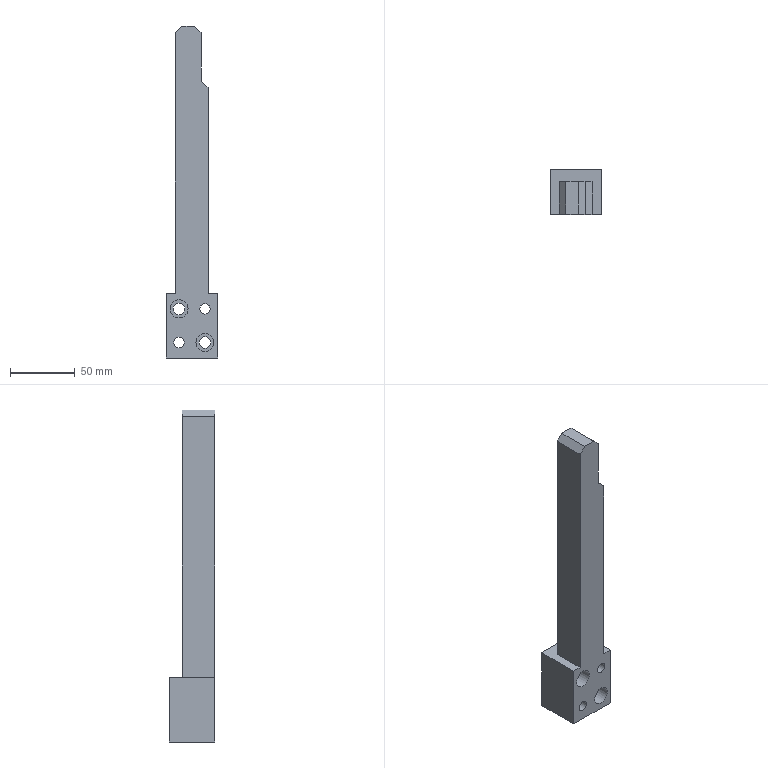Part | STEP file | 车灯-后视镜_id162_x_t | 1 solid | 24 faces | box 40 x 35 x 257 mm | volume 187577 mm3 | plane 16 | cylinder 8 | commonest cylinder face diameters 4 x2 8 x2 9 x2 14 x2
STEP:
#1=CARTESIAN_POINT('',(64.914,-310.,-210.914));
#2=VERTEX_POINT('',#1);
#3=CARTESIAN_POINT('',(60.086,-310.,-206.086));
#4=VERTEX_POINT('',#3);
#5=CARTESIAN_POINT('',(65.5,-310.,-211.5));
#6=DIRECTION('',(-0.7071,0.,0.7071));
#7=VECTOR('',#6,1.);
#8=LINE('',#5,#7);
#9=EDGE_CURVE('',#2,#4,#8,.T.);
#10=ORIENTED_EDGE('',*,*,#9,.F.);
#11=CARTESIAN_POINT('',(64.914,-285.,-210.914));
#12=VERTEX_POINT('',#11);
#13=CARTESIAN_POINT('',(64.914,-285.,-210.914));
#14=DIRECTION('',(0.,1.,0.));
#15=VECTOR('',#14,1.);
#16=LINE('',#13,#15);
#17=EDGE_CURVE('',#2,#12,#16,.T.);
#18=ORIENTED_EDGE('',*,*,#17,.T.);
#19=CARTESIAN_POINT('',(60.086,-285.,-206.086));
#20=VERTEX_POINT('',#19);
#21=CARTESIAN_POINT('',(65.5,-285.,-211.5));
#22=DIRECTION('',(0.7071,0.,-0.7071));
#23=VECTOR('',#22,1.);
#24=LINE('',#21,#23);
#25=EDGE_CURVE('',#20,#12,#24,.T.);
#26=ORIENTED_EDGE('',*,*,#25,.F.);
#27=CARTESIAN_POINT('',(60.086,-310.,-206.086));
#28=DIRECTION('',(0.,-1.,0.));
#29=VECTOR('',#28,1.);
#30=LINE('',#27,#29);
#31=EDGE_CURVE('',#20,#4,#30,.T.);
#32=ORIENTED_EDGE('',*,*,#31,.T.);
#33=EDGE_LOOP('',(#10,#18,#26,#32));
#34=FACE_OUTER_BOUND('',#33,.T.);
#35=CARTESIAN_POINT('',(65.5,-285.,-211.5));
#36=DIRECTION('',(0.7071,0.,0.7071));
#37=DIRECTION('',(0.7071,0.,-0.7071));
#38=AXIS2_PLACEMENT_3D('',#35,#36,#37);
#39=PLANE('',#38);
#40=ADVANCED_FACE('',(#34),#39,.T.);
#41=CARTESIAN_POINT('',(65.5,-285.,-370.5));
#42=VERTEX_POINT('',#41);
#43=CARTESIAN_POINT('',(65.5,-285.,-212.328));
#44=VERTEX_POINT('',#43);
#45=CARTESIAN_POINT('',(65.5,-285.,-420.5));
#46=DIRECTION('',(0.,0.,1.));
#47=VECTOR('',#46,1.);
#48=LINE('',#45,#47);
#49=EDGE_CURVE('',#42,#44,#48,.T.);
#50=ORIENTED_EDGE('',*,*,#49,.T.);
#51=CARTESIAN_POINT('',(65.5,-310.,-212.328));
#52=VERTEX_POINT('',#51);
#53=CARTESIAN_POINT('',(65.5,-292.5,-212.328));
#54=DIRECTION('',(0.,-1.,0.));
#55=VECTOR('',#54,1.);
#56=LINE('',#53,#55);
#57=EDGE_CURVE('',#44,#52,#56,.T.);
#58=ORIENTED_EDGE('',*,*,#57,.T.);
#59=CARTESIAN_POINT('',(65.5,-310.,-370.5));
#60=VERTEX_POINT('',#59);
#61=CARTESIAN_POINT('',(65.5,-310.,-420.5));
#62=DIRECTION('',(0.,0.,1.));
#63=VECTOR('',#62,1.);
#64=LINE('',#61,#63);
#65=EDGE_CURVE('',#60,#52,#64,.T.);
#66=ORIENTED_EDGE('',*,*,#65,.F.);
#67=CARTESIAN_POINT('',(65.5,-292.5,-370.5));
#68=DIRECTION('',(0.,1.,0.));
#69=VECTOR('',#68,1.);
#70=LINE('',#67,#69);
#71=EDGE_CURVE('',#60,#42,#70,.T.);
#72=ORIENTED_EDGE('',*,*,#71,.T.);
#73=EDGE_LOOP('',(#50,#58,#66,#72));
#74=FACE_OUTER_BOUND('',#73,.T.);
#75=CARTESIAN_POINT('',(65.5,-292.5,-420.5));
#76=DIRECTION('',(1.,0.,0.));
#77=DIRECTION('',(0.,0.,-1.));
#78=AXIS2_PLACEMENT_3D('',#75,#76,#77);
#79=PLANE('',#78);
#80=ADVANCED_FACE('',(#74),#79,.T.);
#81=ORIENTED_EDGE('',*,*,#25,.T.);
#82=CARTESIAN_POINT('',(63.5,-285.,-212.328));
#83=DIRECTION('',(0.,1.,0.));
#84=DIRECTION('',(0.,0.,1.));
#85=AXIS2_PLACEMENT_3D('',#82,#83,#84);
#86=CIRCLE('',#85,2.);
#87=EDGE_CURVE('',#12,#44,#86,.T.);
#88=ORIENTED_EDGE('',*,*,#87,.T.);
#89=ORIENTED_EDGE('',*,*,#49,.F.);
#90=CARTESIAN_POINT('',(39.5,-285.,-370.5));
#91=VERTEX_POINT('',#90);
#92=CARTESIAN_POINT('',(52.5,-285.,-370.5));
#93=DIRECTION('',(-1.,0.,0.));
#94=VECTOR('',#93,1.);
#95=LINE('',#92,#94);
#96=EDGE_CURVE('',#42,#91,#95,.T.);
#97=ORIENTED_EDGE('',*,*,#96,.T.);
#98=CARTESIAN_POINT('',(39.5,-285.,-168.5));
#99=VERTEX_POINT('',#98);
#100=CARTESIAN_POINT('',(39.5,-285.,-420.5));
#101=DIRECTION('',(0.,0.,1.));
#102=VECTOR('',#101,1.);
#103=LINE('',#100,#102);
#104=EDGE_CURVE('',#91,#99,#103,.T.);
#105=ORIENTED_EDGE('',*,*,#104,.T.);
#106=CARTESIAN_POINT('',(44.5,-285.,-163.5));
#107=VERTEX_POINT('',#106);
#108=CARTESIAN_POINT('',(39.5,-285.,-168.5));
#109=DIRECTION('',(0.7071,0.,0.7071));
#110=VECTOR('',#109,1.);
#111=LINE('',#108,#110);
#112=EDGE_CURVE('',#99,#107,#111,.T.);
#113=ORIENTED_EDGE('',*,*,#112,.T.);
#114=CARTESIAN_POINT('',(54.5,-285.,-163.5));
#115=VERTEX_POINT('',#114);
#116=CARTESIAN_POINT('',(52.5,-285.,-163.5));
#117=DIRECTION('',(1.,0.,0.));
#118=VECTOR('',#117,1.);
#119=LINE('',#116,#118);
#120=EDGE_CURVE('',#107,#115,#119,.T.);
#121=ORIENTED_EDGE('',*,*,#120,.T.);
#122=CARTESIAN_POINT('',(59.5,-285.,-168.5));
#123=VERTEX_POINT('',#122);
#124=CARTESIAN_POINT('',(59.5,-285.,-168.5));
#125=DIRECTION('',(0.7071,0.,-0.7071));
#126=VECTOR('',#125,1.);
#127=LINE('',#124,#126);
#128=EDGE_CURVE('',#115,#123,#127,.T.);
#129=ORIENTED_EDGE('',*,*,#128,.T.);
#130=CARTESIAN_POINT('',(59.5,-285.,-204.672));
#131=VERTEX_POINT('',#130);
#132=CARTESIAN_POINT('',(59.5,-285.,-420.5));
#133=DIRECTION('',(0.,0.,1.));
#134=VECTOR('',#133,1.);
#135=LINE('',#132,#134);
#136=EDGE_CURVE('',#131,#123,#135,.T.);
#137=ORIENTED_EDGE('',*,*,#136,.F.);
#138=CARTESIAN_POINT('',(61.5,-285.,-204.672));
#139=DIRECTION('',(0.,-1.,0.));
#140=DIRECTION('',(0.,0.,1.));
#141=AXIS2_PLACEMENT_3D('',#138,#139,#140);
#142=CIRCLE('',#141,2.);
#143=EDGE_CURVE('',#131,#20,#142,.T.);
#144=ORIENTED_EDGE('',*,*,#143,.T.);
#145=EDGE_LOOP('',(#81,#88,#89,#97,#105,#113,#121,#129,#137,#144));
#146=FACE_OUTER_BOUND('',#145,.T.);
#147=CARTESIAN_POINT('',(52.5,-285.,-420.5));
#148=DIRECTION('',(0.,1.,0.));
#149=DIRECTION('',(0.,0.,1.));
#150=AXIS2_PLACEMENT_3D('',#147,#148,#149);
#151=PLANE('',#150);
#152=ADVANCED_FACE('',(#146),#151,.T.);
#153=CARTESIAN_POINT('',(39.5,-310.,-370.5));
#154=VERTEX_POINT('',#153);
#155=CARTESIAN_POINT('',(39.5,-310.,-168.5));
#156=VERTEX_POINT('',#155);
#157=CARTESIAN_POINT('',(39.5,-310.,-420.5));
#158=DIRECTION('',(0.,0.,1.));
#159=VECTOR('',#158,1.);
#160=LINE('',#157,#159);
#161=EDGE_CURVE('',#154,#156,#160,.T.);
#162=ORIENTED_EDGE('',*,*,#161,.T.);
#163=CARTESIAN_POINT('',(39.5,-292.5,-168.5));
#164=DIRECTION('',(0.,1.,0.));
#165=VECTOR('',#164,1.);
#166=LINE('',#163,#165);
#167=EDGE_CURVE('',#156,#99,#166,.T.);
#168=ORIENTED_EDGE('',*,*,#167,.T.);
#169=ORIENTED_EDGE('',*,*,#104,.F.);
#170=CARTESIAN_POINT('',(39.5,-292.5,-370.5));
#171=DIRECTION('',(0.,-1.,0.));
#172=VECTOR('',#171,1.);
#173=LINE('',#170,#172);
#174=EDGE_CURVE('',#91,#154,#173,.T.);
#175=ORIENTED_EDGE('',*,*,#174,.T.);
#176=EDGE_LOOP('',(#162,#168,#169,#175));
#177=FACE_OUTER_BOUND('',#176,.T.);
#178=CARTESIAN_POINT('',(39.5,-292.5,-420.5));
#179=DIRECTION('',(-1.,0.,0.));
#180=DIRECTION('',(0.,0.,1.));
#181=AXIS2_PLACEMENT_3D('',#178,#179,#180);
#182=PLANE('',#181);
#183=ADVANCED_FACE('',(#177),#182,.T.);
#184=CARTESIAN_POINT('',(55.5,-310.,-408.5));
#185=VERTEX_POINT('',#184);
#186=CARTESIAN_POINT('',(62.5,-310.,-408.5));
#187=DIRECTION('',(0.,1.,0.));
#188=DIRECTION('',(-1.,0.,0.));
#189=AXIS2_PLACEMENT_3D('',#186,#187,#188);
#190=CIRCLE('',#189,7.);
#191=EDGE_CURVE('',#185,#185,#190,.T.);
#192=ORIENTED_EDGE('',*,*,#191,.T.);
#193=EDGE_LOOP('',(#192));
#194=FACE_BOUND('',#193,.T.);
#195=CARTESIAN_POINT('',(35.5,-310.,-382.5));
#196=VERTEX_POINT('',#195);
#197=CARTESIAN_POINT('',(42.5,-310.,-382.5));
#198=DIRECTION('',(0.,1.,0.));
#199=DIRECTION('',(-1.,0.,0.));
#200=AXIS2_PLACEMENT_3D('',#197,#198,#199);
#201=CIRCLE('',#200,7.);
#202=EDGE_CURVE('',#196,#196,#201,.T.);
#203=ORIENTED_EDGE('',*,*,#202,.T.);
#204=EDGE_LOOP('',(#203));
#205=FACE_BOUND('',#204,.T.);
#206=CARTESIAN_POINT('',(42.5,-310.,-404.5));
#207=VERTEX_POINT('',#206);
#208=CARTESIAN_POINT('',(42.5,-310.,-408.5));
#209=DIRECTION('',(0.,1.,0.));
#210=DIRECTION('',(0.,0.,1.));
#211=AXIS2_PLACEMENT_3D('',#208,#209,#210);
#212=CIRCLE('',#211,4.);
#213=EDGE_CURVE('',#207,#207,#212,.T.);
#214=ORIENTED_EDGE('',*,*,#213,.T.);
#215=EDGE_LOOP('',(#214));
#216=FACE_BOUND('',#215,.T.);
#217=CARTESIAN_POINT('',(62.5,-310.,-378.5));
#218=VERTEX_POINT('',#217);
#219=CARTESIAN_POINT('',(62.5,-310.,-382.5));
#220=DIRECTION('',(0.,1.,0.));
#221=DIRECTION('',(0.,0.,1.));
#222=AXIS2_PLACEMENT_3D('',#219,#220,#221);
#223=CIRCLE('',#222,4.);
#224=EDGE_CURVE('',#218,#218,#223,.T.);
#225=ORIENTED_EDGE('',*,*,#224,.T.);
#226=EDGE_LOOP('',(#225));
#227=FACE_BOUND('',#226,.T.);
#228=ORIENTED_EDGE('',*,*,#65,.T.);
#229=CARTESIAN_POINT('',(63.5,-310.,-212.328));
#230=DIRECTION('',(0.,-1.,0.));
#231=DIRECTION('',(0.,0.,-1.));
#232=AXIS2_PLACEMENT_3D('',#229,#230,#231);
#233=CIRCLE('',#232,2.);
#234=EDGE_CURVE('',#52,#2,#233,.T.);
#235=ORIENTED_EDGE('',*,*,#234,.T.);
#236=ORIENTED_EDGE('',*,*,#9,.T.);
#237=CARTESIAN_POINT('',(59.5,-310.,-204.672));
#238=VERTEX_POINT('',#237);
#239=CARTESIAN_POINT('',(61.5,-310.,-204.672));
#240=DIRECTION('',(0.,1.,0.));
#241=DIRECTION('',(0.,0.,-1.));
#242=AXIS2_PLACEMENT_3D('',#239,#240,#241);
#243=CIRCLE('',#242,2.);
#244=EDGE_CURVE('',#4,#238,#243,.T.);
#245=ORIENTED_EDGE('',*,*,#244,.T.);
#246=CARTESIAN_POINT('',(59.5,-310.,-168.5));
#247=VERTEX_POINT('',#246);
#248=CARTESIAN_POINT('',(59.5,-310.,-433.5));
#249=DIRECTION('',(0.,0.,1.));
#250=VECTOR('',#249,1.);
#251=LINE('',#248,#250);
#252=EDGE_CURVE('',#238,#247,#251,.T.);
#253=ORIENTED_EDGE('',*,*,#252,.T.);
#254=CARTESIAN_POINT('',(54.5,-310.,-163.5));
#255=VERTEX_POINT('',#254);
#256=CARTESIAN_POINT('',(59.5,-310.,-168.5));
#257=DIRECTION('',(-0.7071,0.,0.7071));
#258=VECTOR('',#257,1.);
#259=LINE('',#256,#258);
#260=EDGE_CURVE('',#247,#255,#259,.T.);
#261=ORIENTED_EDGE('',*,*,#260,.T.);
#262=CARTESIAN_POINT('',(44.5,-310.,-163.5));
#263=VERTEX_POINT('',#262);
#264=CARTESIAN_POINT('',(52.5,-310.,-163.5));
#265=DIRECTION('',(-1.,0.,0.));
#266=VECTOR('',#265,1.);
#267=LINE('',#264,#266);
#268=EDGE_CURVE('',#255,#263,#267,.T.);
#269=ORIENTED_EDGE('',*,*,#268,.T.);
#270=CARTESIAN_POINT('',(39.5,-310.,-168.5));
#271=DIRECTION('',(-0.7071,0.,-0.7071));
#272=VECTOR('',#271,1.);
#273=LINE('',#270,#272);
#274=EDGE_CURVE('',#263,#156,#273,.T.);
#275=ORIENTED_EDGE('',*,*,#274,.T.);
#276=ORIENTED_EDGE('',*,*,#161,.F.);
#277=CARTESIAN_POINT('',(32.5,-310.,-370.5));
#278=VERTEX_POINT('',#277);
#279=CARTESIAN_POINT('',(52.5,-310.,-370.5));
#280=DIRECTION('',(1.,0.,0.));
#281=VECTOR('',#280,1.);
#282=LINE('',#279,#281);
#283=EDGE_CURVE('',#278,#154,#282,.T.);
#284=ORIENTED_EDGE('',*,*,#283,.F.);
#285=CARTESIAN_POINT('',(32.5,-310.,-420.5));
#286=VERTEX_POINT('',#285);
#287=CARTESIAN_POINT('',(32.5,-310.,-420.5));
#288=DIRECTION('',(0.,0.,1.));
#289=VECTOR('',#288,1.);
#290=LINE('',#287,#289);
#291=EDGE_CURVE('',#286,#278,#290,.T.);
#292=ORIENTED_EDGE('',*,*,#291,.F.);
#293=CARTESIAN_POINT('',(72.5,-310.,-420.5));
#294=VERTEX_POINT('',#293);
#295=CARTESIAN_POINT('',(52.5,-310.,-420.5));
#296=DIRECTION('',(1.,0.,0.));
#297=VECTOR('',#296,1.);
#298=LINE('',#295,#297);
#299=EDGE_CURVE('',#286,#294,#298,.T.);
#300=ORIENTED_EDGE('',*,*,#299,.T.);
#301=CARTESIAN_POINT('',(72.5,-310.,-370.5));
#302=VERTEX_POINT('',#301);
#303=CARTESIAN_POINT('',(72.5,-310.,-420.5));
#304=DIRECTION('',(0.,0.,1.));
#305=VECTOR('',#304,1.);
#306=LINE('',#303,#305);
#307=EDGE_CURVE('',#294,#302,#306,.T.);
#308=ORIENTED_EDGE('',*,*,#307,.T.);
#309=CARTESIAN_POINT('',(52.5,-310.,-370.5));
#310=DIRECTION('',(1.,0.,0.));
#311=VECTOR('',#310,1.);
#312=LINE('',#309,#311);
#313=EDGE_CURVE('',#60,#302,#312,.T.);
#314=ORIENTED_EDGE('',*,*,#313,.F.);
#315=EDGE_LOOP('',(#228,#235,#236,#245,#253,#261,#269,#275,#276,#284,#292,#300,#308,#314));
#316=FACE_BOUND('',#315,.T.);
#317=CARTESIAN_POINT('',(52.5,-310.,-420.5));
#318=DIRECTION('',(0.,-1.,0.));
#319=DIRECTION('',(0.,0.,-1.));
#320=AXIS2_PLACEMENT_3D('',#317,#318,#319);
#321=PLANE('',#320);
#322=ADVANCED_FACE('',(#194,#205,#216,#227,#316),#321,.T.);
#323=CARTESIAN_POINT('',(32.5,-275.,-370.5));
#324=VERTEX_POINT('',#323);
#325=CARTESIAN_POINT('',(32.5,-292.5,-370.5));
#326=DIRECTION('',(0.,-1.,0.));
#327=VECTOR('',#326,1.);
#328=LINE('',#325,#327);
#329=EDGE_CURVE('',#324,#278,#328,.T.);
#330=ORIENTED_EDGE('',*,*,#329,.F.);
#331=CARTESIAN_POINT('',(32.5,-275.,-420.5));
#332=VERTEX_POINT('',#331);
#333=CARTESIAN_POINT('',(32.5,-275.,-420.5));
#334=DIRECTION('',(0.,0.,1.));
#335=VECTOR('',#334,1.);
#336=LINE('',#333,#335);
#337=EDGE_CURVE('',#332,#324,#336,.T.);
#338=ORIENTED_EDGE('',*,*,#337,.F.);
#339=CARTESIAN_POINT('',(32.5,-292.5,-420.5));
#340=DIRECTION('',(0.,-1.,0.));
#341=VECTOR('',#340,1.);
#342=LINE('',#339,#341);
#343=EDGE_CURVE('',#332,#286,#342,.T.);
#344=ORIENTED_EDGE('',*,*,#343,.T.);
#345=ORIENTED_EDGE('',*,*,#291,.T.);
#346=EDGE_LOOP('',(#330,#338,#344,#345));
#347=FACE_OUTER_BOUND('',#346,.T.);
#348=CARTESIAN_POINT('',(32.5,-292.5,-420.5));
#349=DIRECTION('',(-1.,0.,0.));
#350=DIRECTION('',(0.,0.,1.));
#351=AXIS2_PLACEMENT_3D('',#348,#349,#350);
#352=PLANE('',#351);
#353=ADVANCED_FACE('',(#347),#352,.T.);
#354=CARTESIAN_POINT('',(42.5,-275.,-404.5));
#355=VERTEX_POINT('',#354);
#356=CARTESIAN_POINT('',(42.5,-275.,-408.5));
#357=DIRECTION('',(0.,1.,0.));
#358=DIRECTION('',(0.,0.,1.));
#359=AXIS2_PLACEMENT_3D('',#356,#357,#358);
#360=CIRCLE('',#359,4.);
#361=EDGE_CURVE('',#355,#355,#360,.T.);
#362=ORIENTED_EDGE('',*,*,#361,.F.);
#363=EDGE_LOOP('',(#362));
#364=FACE_BOUND('',#363,.T.);
#365=CARTESIAN_POINT('',(62.5,-275.,-404.));
#366=VERTEX_POINT('',#365);
#367=CARTESIAN_POINT('',(62.5,-275.,-408.5));
#368=DIRECTION('',(0.,1.,0.));
#369=DIRECTION('',(0.,0.,1.));
#370=AXIS2_PLACEMENT_3D('',#367,#368,#369);
#371=CIRCLE('',#370,4.5);
#372=EDGE_CURVE('',#366,#366,#371,.T.);
#373=ORIENTED_EDGE('',*,*,#372,.F.);
#374=EDGE_LOOP('',(#373));
#375=FACE_BOUND('',#374,.T.);
#376=CARTESIAN_POINT('',(62.5,-275.,-378.5));
#377=VERTEX_POINT('',#376);
#378=CARTESIAN_POINT('',(62.5,-275.,-382.5));
#379=DIRECTION('',(0.,1.,0.));
#380=DIRECTION('',(0.,0.,1.));
#381=AXIS2_PLACEMENT_3D('',#378,#379,#380);
#382=CIRCLE('',#381,4.);
#383=EDGE_CURVE('',#377,#377,#382,.T.);
#384=ORIENTED_EDGE('',*,*,#383,.F.);
#385=EDGE_LOOP('',(#384));
#386=FACE_BOUND('',#385,.T.);
#387=CARTESIAN_POINT('',(42.5,-275.,-378.));
#388=VERTEX_POINT('',#387);
#389=CARTESIAN_POINT('',(42.5,-275.,-382.5));
#390=DIRECTION('',(0.,1.,0.));
#391=DIRECTION('',(0.,0.,1.));
#392=AXIS2_PLACEMENT_3D('',#389,#390,#391);
#393=CIRCLE('',#392,4.5);
#394=EDGE_CURVE('',#388,#388,#393,.T.);
#395=ORIENTED_EDGE('',*,*,#394,.F.);
#396=EDGE_LOOP('',(#395));
#397=FACE_BOUND('',#396,.T.);
#398=CARTESIAN_POINT('',(72.5,-275.,-370.5));
#399=VERTEX_POINT('',#398);
#400=CARTESIAN_POINT('',(52.5,-275.,-370.5));
#401=DIRECTION('',(-1.,0.,0.));
#402=VECTOR('',#401,1.);
#403=LINE('',#400,#402);
#404=EDGE_CURVE('',#399,#324,#403,.T.);
#405=ORIENTED_EDGE('',*,*,#404,.F.);
#406=CARTESIAN_POINT('',(72.5,-275.,-420.5));
#407=VERTEX_POINT('',#406);
#408=CARTESIAN_POINT('',(72.5,-275.,-420.5));
#409=DIRECTION('',(0.,0.,1.));
#410=VECTOR('',#409,1.);
#411=LINE('',#408,#410);
#412=EDGE_CURVE('',#407,#399,#411,.T.);
#413=ORIENTED_EDGE('',*,*,#412,.F.);
#414=CARTESIAN_POINT('',(52.5,-275.,-420.5));
#415=DIRECTION('',(-1.,0.,0.));
#416=VECTOR('',#415,1.);
#417=LINE('',#414,#416);
#418=EDGE_CURVE('',#407,#332,#417,.T.);
#419=ORIENTED_EDGE('',*,*,#418,.T.);
#420=ORIENTED_EDGE('',*,*,#337,.T.);
#421=EDGE_LOOP('',(#405,#413,#419,#420));
#422=FACE_BOUND('',#421,.T.);
#423=CARTESIAN_POINT('',(52.5,-275.,-420.5));
#424=DIRECTION('',(0.,1.,0.));
#425=DIRECTION('',(0.,0.,1.));
#426=AXIS2_PLACEMENT_3D('',#423,#424,#425);
#427=PLANE('',#426);
#428=ADVANCED_FACE('',(#364,#375,#386,#397,#422),#427,.T.);
#429=CARTESIAN_POINT('',(72.5,-292.5,-420.5));
#430=DIRECTION('',(0.,1.,0.));
#431=VECTOR('',#430,1.);
#432=LINE('',#429,#431);
#433=EDGE_CURVE('',#294,#407,#432,.T.);
#434=ORIENTED_EDGE('',*,*,#433,.F.);
#435=ORIENTED_EDGE('',*,*,#299,.F.);
#436=ORIENTED_EDGE('',*,*,#343,.F.);
#437=ORIENTED_EDGE('',*,*,#418,.F.);
#438=EDGE_LOOP('',(#434,#435,#436,#437));
#439=FACE_OUTER_BOUND('',#438,.T.);
#440=CARTESIAN_POINT('',(52.5,-292.5,-420.5));
#441=DIRECTION('',(0.,0.,-1.));
#442=DIRECTION('',(-1.,0.,0.));
#443=AXIS2_PLACEMENT_3D('',#440,#441,#442);
#444=PLANE('',#443);
#445=ADVANCED_FACE('',(#439),#444,.T.);
#446=CARTESIAN_POINT('',(72.5,-292.5,-370.5));
#447=DIRECTION('',(0.,1.,0.));
#448=VECTOR('',#447,1.);
#449=LINE('',#446,#448);
#450=EDGE_CURVE('',#302,#399,#449,.T.);
#451=ORIENTED_EDGE('',*,*,#450,.F.);
#452=ORIENTED_EDGE('',*,*,#307,.F.);
#453=ORIENTED_EDGE('',*,*,#433,.T.);
#454=ORIENTED_EDGE('',*,*,#412,.T.);
#455=EDGE_LOOP('',(#451,#452,#453,#454));
#456=FACE_OUTER_BOUND('',#455,.T.);
#457=CARTESIAN_POINT('',(72.5,-292.5,-420.5));
#458=DIRECTION('',(1.,0.,0.));
#459=DIRECTION('',(0.,0.,-1.));
#460=AXIS2_PLACEMENT_3D('',#457,#458,#459);
#461=PLANE('',#460);
#462=ADVANCED_FACE('',(#456),#461,.T.);
#463=ORIENTED_EDGE('',*,*,#174,.F.);
#464=ORIENTED_EDGE('',*,*,#96,.F.);
#465=ORIENTED_EDGE('',*,*,#71,.F.);
#466=ORIENTED_EDGE('',*,*,#313,.T.);
#467=ORIENTED_EDGE('',*,*,#450,.T.);
#468=ORIENTED_EDGE('',*,*,#404,.T.);
#469=ORIENTED_EDGE('',*,*,#329,.T.);
#470=ORIENTED_EDGE('',*,*,#283,.T.);
#471=EDGE_LOOP('',(#463,#464,#465,#466,#467,#468,#469,#470));
#472=FACE_OUTER_BOUND('',#471,.T.);
#473=CARTESIAN_POINT('',(52.5,-292.5,-370.5));
#474=DIRECTION('',(0.,0.,-1.));
#475=DIRECTION('',(-1.,0.,0.));
#476=AXIS2_PLACEMENT_3D('',#473,#474,#475);
#477=PLANE('',#476);
#478=ADVANCED_FACE('',(#472),#477,.F.);
#479=ORIENTED_EDGE('',*,*,#268,.F.);
#480=CARTESIAN_POINT('',(54.5,-292.5,-163.5));
#481=DIRECTION('',(0.,1.,0.));
#482=VECTOR('',#481,1.);
#483=LINE('',#480,#482);
#484=EDGE_CURVE('',#255,#115,#483,.T.);
#485=ORIENTED_EDGE('',*,*,#484,.T.);
#486=ORIENTED_EDGE('',*,*,#120,.F.);
#487=CARTESIAN_POINT('',(44.5,-292.5,-163.5));
#488=DIRECTION('',(0.,-1.,0.));
#489=VECTOR('',#488,1.);
#490=LINE('',#487,#489);
#491=EDGE_CURVE('',#107,#263,#490,.T.);
#492=ORIENTED_EDGE('',*,*,#491,.T.);
#493=EDGE_LOOP('',(#479,#485,#486,#492));
#494=FACE_OUTER_BOUND('',#493,.T.);
#495=CARTESIAN_POINT('',(52.5,-292.5,-163.5));
#496=DIRECTION('',(0.,0.,1.));
#497=DIRECTION('',(1.,0.,0.));
#498=AXIS2_PLACEMENT_3D('',#495,#496,#497);
#499=PLANE('',#498);
#500=ADVANCED_FACE('',(#494),#499,.T.);
#501=ORIENTED_EDGE('',*,*,#252,.F.);
#502=CARTESIAN_POINT('',(59.5,-285.,-204.672));
#503=DIRECTION('',(0.,1.,0.));
#504=VECTOR('',#503,1.);
#505=LINE('',#502,#504);
#506=EDGE_CURVE('',#238,#131,#505,.T.);
#507=ORIENTED_EDGE('',*,*,#506,.T.);
#508=ORIENTED_EDGE('',*,*,#136,.T.);
#509=CARTESIAN_POINT('',(59.5,-292.5,-168.5));
#510=DIRECTION('',(0.,-1.,0.));
#511=VECTOR('',#510,1.);
#512=LINE('',#509,#511);
#513=EDGE_CURVE('',#123,#247,#512,.T.);
#514=ORIENTED_EDGE('',*,*,#513,.T.);
#515=EDGE_LOOP('',(#501,#507,#508,#514));
#516=FACE_OUTER_BOUND('',#515,.T.);
#517=CARTESIAN_POINT('',(59.5,-292.5,-433.5));
#518=DIRECTION('',(1.,0.,0.));
#519=DIRECTION('',(0.,0.,-1.));
#520=AXIS2_PLACEMENT_3D('',#517,#518,#519);
#521=PLANE('',#520);
#522=ADVANCED_FACE('',(#516),#521,.T.);
#523=ORIENTED_EDGE('',*,*,#128,.F.);
#524=ORIENTED_EDGE('',*,*,#484,.F.);
#525=ORIENTED_EDGE('',*,*,#260,.F.);
#526=ORIENTED_EDGE('',*,*,#513,.F.);
#527=EDGE_LOOP('',(#523,#524,#525,#526));
#528=FACE_OUTER_BOUND('',#527,.T.);
#529=CARTESIAN_POINT('',(59.5,-292.5,-168.5));
#530=DIRECTION('',(-0.7071,0.,-0.7071));
#531=DIRECTION('',(-0.7071,0.,0.7071));
#532=AXIS2_PLACEMENT_3D('',#529,#530,#531);
#533=PLANE('',#532);
#534=ADVANCED_FACE('',(#528),#533,.F.);
#535=ORIENTED_EDGE('',*,*,#274,.F.);
#536=ORIENTED_EDGE('',*,*,#491,.F.);
#537=ORIENTED_EDGE('',*,*,#112,.F.);
#538=ORIENTED_EDGE('',*,*,#167,.F.);
#539=EDGE_LOOP('',(#535,#536,#537,#538));
#540=FACE_OUTER_BOUND('',#539,.T.);
#541=CARTESIAN_POINT('',(39.5,-292.5,-168.5));
#542=DIRECTION('',(0.7071,0.,-0.7071));
#543=DIRECTION('',(-0.7071,0.,-0.7071));
#544=AXIS2_PLACEMENT_3D('',#541,#542,#543);
#545=PLANE('',#544);
#546=ADVANCED_FACE('',(#540),#545,.F.);
#547=ORIENTED_EDGE('',*,*,#87,.F.);
#548=ORIENTED_EDGE('',*,*,#17,.F.);
#549=ORIENTED_EDGE('',*,*,#234,.F.);
#550=ORIENTED_EDGE('',*,*,#57,.F.);
#551=EDGE_LOOP('',(#547,#548,#549,#550));
#552=FACE_OUTER_BOUND('',#551,.T.);
#553=CARTESIAN_POINT('',(63.5,-292.5,-212.328));
#554=DIRECTION('',(0.,-1.,0.));
#555=DIRECTION('',(0.,0.,-1.));
#556=AXIS2_PLACEMENT_3D('',#553,#554,#555);
#557=CYLINDRICAL_SURFACE('',#556,2.);
#558=ADVANCED_FACE('',(#552),#557,.T.);
#559=ORIENTED_EDGE('',*,*,#143,.F.);
#560=ORIENTED_EDGE('',*,*,#506,.F.);
#561=ORIENTED_EDGE('',*,*,#244,.F.);
#562=ORIENTED_EDGE('',*,*,#31,.F.);
#563=EDGE_LOOP('',(#559,#560,#561,#562));
#564=FACE_OUTER_BOUND('',#563,.T.);
#565=CARTESIAN_POINT('',(61.5,-285.,-204.672));
#566=DIRECTION('',(0.,1.,0.));
#567=DIRECTION('',(0.,0.,1.));
#568=AXIS2_PLACEMENT_3D('',#565,#566,#567);
#569=CYLINDRICAL_SURFACE('',#568,2.);
#570=ADVANCED_FACE('',(#564),#569,.F.);
#571=CARTESIAN_POINT('',(42.5,-301.,-378.));
#572=VERTEX_POINT('',#571);
#573=CARTESIAN_POINT('',(42.5,-301.,-382.5));
#574=DIRECTION('',(0.,-1.,0.));
#575=DIRECTION('',(0.,0.,1.));
#576=AXIS2_PLACEMENT_3D('',#573,#574,#575);
#577=CIRCLE('',#576,4.5);
#578=EDGE_CURVE('',#572,#572,#577,.T.);
#579=ORIENTED_EDGE('',*,*,#578,.T.);
#580=EDGE_LOOP('',(#579));
#581=FACE_BOUND('',#580,.T.);
#582=ORIENTED_EDGE('',*,*,#394,.T.);
#583=EDGE_LOOP('',(#582));
#584=FACE_BOUND('',#583,.T.);
#585=CARTESIAN_POINT('',(42.5,-310.,-382.5));
#586=DIRECTION('',(0.,1.,0.));
#587=DIRECTION('',(0.,0.,1.));
#588=AXIS2_PLACEMENT_3D('',#585,#586,#587);
#589=CYLINDRICAL_SURFACE('',#588,4.5);
#590=ADVANCED_FACE('',(#581,#584),#589,.F.);
#591=ORIENTED_EDGE('',*,*,#383,.T.);
#592=EDGE_LOOP('',(#591));
#593=FACE_BOUND('',#592,.T.);
#594=ORIENTED_EDGE('',*,*,#224,.F.);
#595=EDGE_LOOP('',(#594));
#596=FACE_BOUND('',#595,.T.);
#597=CARTESIAN_POINT('',(62.5,-310.,-382.5));
#598=DIRECTION('',(0.,1.,0.));
#599=DIRECTION('',(0.,0.,1.));
#600=AXIS2_PLACEMENT_3D('',#597,#598,#599);
#601=CYLINDRICAL_SURFACE('',#600,4.);
#602=ADVANCED_FACE('',(#593,#596),#601,.F.);
#603=CARTESIAN_POINT('',(62.5,-301.,-404.));
#604=VERTEX_POINT('',#603);
#605=CARTESIAN_POINT('',(62.5,-301.,-408.5));
#606=DIRECTION('',(0.,-1.,0.));
#607=DIRECTION('',(0.,0.,1.));
#608=AXIS2_PLACEMENT_3D('',#605,#606,#607);
#609=CIRCLE('',#608,4.5);
#610=EDGE_CURVE('',#604,#604,#609,.T.);
#611=ORIENTED_EDGE('',*,*,#610,.T.);
#612=EDGE_LOOP('',(#611));
#613=FACE_BOUND('',#612,.T.);
#614=ORIENTED_EDGE('',*,*,#372,.T.);
#615=EDGE_LOOP('',(#614));
#616=FACE_BOUND('',#615,.T.);
#617=CARTESIAN_POINT('',(62.5,-310.,-408.5));
#618=DIRECTION('',(0.,1.,0.));
#619=DIRECTION('',(0.,0.,1.));
#620=AXIS2_PLACEMENT_3D('',#617,#618,#619);
#621=CYLINDRICAL_SURFACE('',#620,4.5);
#622=ADVANCED_FACE('',(#613,#616),#621,.F.);
#623=ORIENTED_EDGE('',*,*,#361,.T.);
#624=EDGE_LOOP('',(#623));
#625=FACE_BOUND('',#624,.T.);
#626=ORIENTED_EDGE('',*,*,#213,.F.);
#627=EDGE_LOOP('',(#626));
#628=FACE_BOUND('',#627,.T.);
#629=CARTESIAN_POINT('',(42.5,-310.,-408.5));
#630=DIRECTION('',(0.,1.,0.));
#631=DIRECTION('',(0.,0.,1.));
#632=AXIS2_PLACEMENT_3D('',#629,#630,#631);
#633=CYLINDRICAL_SURFACE('',#632,4.);
#634=ADVANCED_FACE('',(#625,#628),#633,.F.);
#635=ORIENTED_EDGE('',*,*,#578,.F.);
#636=EDGE_LOOP('',(#635));
#637=FACE_BOUND('',#636,.T.);
#638=CARTESIAN_POINT('',(49.5,-301.,-382.5));
#639=VERTEX_POINT('',#638);
#640=CARTESIAN_POINT('',(42.5,-301.,-382.5));
#641=DIRECTION('',(0.,-1.,0.));
#642=DIRECTION('',(1.,0.,0.));
#643=AXIS2_PLACEMENT_3D('',#640,#641,#642);
#644=CIRCLE('',#643,7.);
#645=EDGE_CURVE('',#639,#639,#644,.T.);
#646=ORIENTED_EDGE('',*,*,#645,.T.);
#647=EDGE_LOOP('',(#646));
#648=FACE_BOUND('',#647,.T.);
#649=CARTESIAN_POINT('',(42.5,-301.,-382.5));
#650=DIRECTION('',(0.,1.,0.));
#651=DIRECTION('',(-1.,0.,0.));
#652=AXIS2_PLACEMENT_3D('',#649,#650,#651);
#653=PLANE('',#652);
#654=ADVANCED_FACE('',(#637,#648),#653,.F.);
#655=ORIENTED_EDGE('',*,*,#645,.F.);
#656=EDGE_LOOP('',(#655));
#657=FACE_BOUND('',#656,.T.);
#658=ORIENTED_EDGE('',*,*,#202,.F.);
#659=EDGE_LOOP('',(#658));
#660=FACE_BOUND('',#659,.T.);
#661=CARTESIAN_POINT('',(42.5,-310.,-382.5));
#662=DIRECTION('',(0.,1.,0.));
#663=DIRECTION('',(-1.,0.,0.));
#664=AXIS2_PLACEMENT_3D('',#661,#662,#663);
#665=CYLINDRICAL_SURFACE('',#664,7.);
#666=ADVANCED_FACE('',(#657,#660),#665,.F.);
#667=ORIENTED_EDGE('',*,*,#610,.F.);
#668=EDGE_LOOP('',(#667));
#669=FACE_BOUND('',#668,.T.);
#670=CARTESIAN_POINT('',(69.5,-301.,-408.5));
#671=VERTEX_POINT('',#670);
#672=CARTESIAN_POINT('',(62.5,-301.,-408.5));
#673=DIRECTION('',(0.,-1.,0.));
#674=DIRECTION('',(1.,0.,0.));
#675=AXIS2_PLACEMENT_3D('',#672,#673,#674);
#676=CIRCLE('',#675,7.);
#677=EDGE_CURVE('',#671,#671,#676,.T.);
#678=ORIENTED_EDGE('',*,*,#677,.T.);
#679=EDGE_LOOP('',(#678));
#680=FACE_BOUND('',#679,.T.);
#681=CARTESIAN_POINT('',(62.5,-301.,-408.5));
#682=DIRECTION('',(0.,1.,0.));
#683=DIRECTION('',(-1.,0.,0.));
#684=AXIS2_PLACEMENT_3D('',#681,#682,#683);
#685=PLANE('',#684);
#686=ADVANCED_FACE('',(#669,#680),#685,.F.);
#687=ORIENTED_EDGE('',*,*,#677,.F.);
#688=EDGE_LOOP('',(#687));
#689=FACE_BOUND('',#688,.T.);
#690=ORIENTED_EDGE('',*,*,#191,.F.);
#691=EDGE_LOOP('',(#690));
#692=FACE_BOUND('',#691,.T.);
#693=CARTESIAN_POINT('',(62.5,-310.,-408.5));
#694=DIRECTION('',(0.,1.,0.));
#695=DIRECTION('',(-1.,0.,0.));
#696=AXIS2_PLACEMENT_3D('',#693,#694,#695);
#697=CYLINDRICAL_SURFACE('',#696,7.);
#698=ADVANCED_FACE('',(#689,#692),#697,.F.);
#699=CLOSED_SHELL('',(#40,#80,#152,#183,#322,#353,#428,#445,#462,#478,#500,#522,#534,#546,#558,#570,#590,#602,#622,#634,#654,#666,#686,#698));
#700=MANIFOLD_SOLID_BREP('',#699);
#701=(LENGTH_UNIT()NAMED_UNIT(*)SI_UNIT(.MILLI.,.METRE.));
#702=UNCERTAINTY_MEASURE_WITH_UNIT(LENGTH_MEASURE(0.00002),#701,'','');
#703=(NAMED_UNIT(*)PLANE_ANGLE_UNIT()SI_UNIT($,.RADIAN.));
#704=PLANE_ANGLE_MEASURE_WITH_UNIT(PLANE_ANGLE_MEASURE(0.01745),#703);
#705=DIMENSIONAL_EXPONENTS(0.,0.,0.,0.,0.,0.,0.);
#706=(CONVERSION_BASED_UNIT('DEGREE',#704)NAMED_UNIT(#705)PLANE_ANGLE_UNIT());
#707=(NAMED_UNIT(*)SI_UNIT($,.STERADIAN.)SOLID_ANGLE_UNIT());
#708=(GEOMETRIC_REPRESENTATION_CONTEXT(3)GLOBAL_UNCERTAINTY_ASSIGNED_CONTEXT((#702))GLOBAL_UNIT_ASSIGNED_CONTEXT((#701,#706,#707))REPRESENTATION_CONTEXT('',''));
#709=ADVANCED_BREP_SHAPE_REPRESENTATION('',(#700),#708);